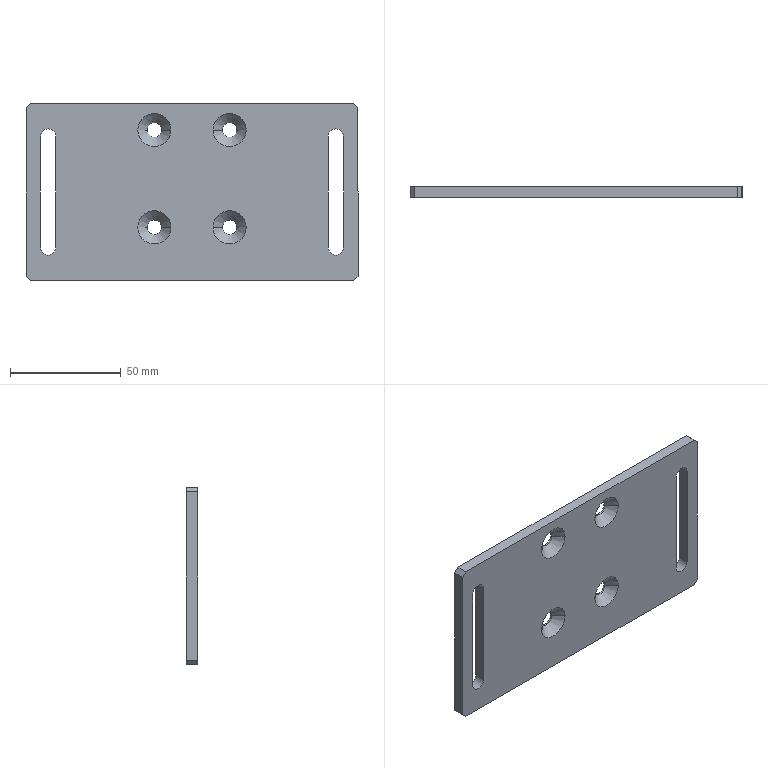Part | SolidWorks | features BaseBody 1 | 1 solid | 36 faces | box 150 x 5 x 80 mm | volume 54349 mm3 | cylinder 14 | plane 14 | cone 8 | commonest cylinder face diameters 6.6 x8 7 x6
STEP:
#1=CARTESIAN_POINT('',(10.,-5.,-11.5));
#2=VERTEX_POINT('',#1);
#3=CARTESIAN_POINT('',(13.5,-5.,-15.));
#4=VERTEX_POINT('',#3);
#5=CARTESIAN_POINT('',(10.,-5.,-15.));
#6=DIRECTION('',(0.,1.,0.));
#7=DIRECTION('',(0.,0.,1.));
#8=AXIS2_PLACEMENT_3D('',#5,#6,#7);
#9=CIRCLE('',#8,3.5);
#10=EDGE_CURVE('',#2,#4,#9,.T.);
#11=ORIENTED_EDGE('',*,*,#10,.F.);
#12=CARTESIAN_POINT('',(10.,0.,-11.5));
#13=VERTEX_POINT('',#12);
#14=CARTESIAN_POINT('',(10.,-10.,-11.5));
#15=DIRECTION('',(0.,1.,0.));
#16=VECTOR('',#15,1000.);
#17=LINE('',#14,#16);
#18=EDGE_CURVE('',#2,#13,#17,.T.);
#19=ORIENTED_EDGE('',*,*,#18,.T.);
#20=CARTESIAN_POINT('',(13.5,0.,-15.));
#21=VERTEX_POINT('',#20);
#22=CARTESIAN_POINT('',(10.,0.,-15.));
#23=DIRECTION('',(0.,1.,0.));
#24=DIRECTION('',(0.,0.,1.));
#25=AXIS2_PLACEMENT_3D('',#22,#23,#24);
#26=CIRCLE('',#25,3.5);
#27=EDGE_CURVE('',#13,#21,#26,.T.);
#28=ORIENTED_EDGE('',*,*,#27,.T.);
#29=CARTESIAN_POINT('',(13.5,-10.,-15.));
#30=DIRECTION('',(0.,-1.,0.));
#31=VECTOR('',#30,1000.);
#32=LINE('',#29,#31);
#33=EDGE_CURVE('',#21,#4,#32,.T.);
#34=ORIENTED_EDGE('',*,*,#33,.T.);
#35=EDGE_LOOP('',(#11,#19,#28,#34));
#36=FACE_OUTER_BOUND('',#35,.T.);
#37=CARTESIAN_POINT('',(10.,-10.,-15.));
#38=DIRECTION('',(0.,1.,0.));
#39=DIRECTION('',(0.,0.,1.));
#40=AXIS2_PLACEMENT_3D('',#37,#38,#39);
#41=CYLINDRICAL_SURFACE('',#40,3.5);
#42=ADVANCED_FACE('',(#36),#41,.F.);
#43=CARTESIAN_POINT('',(140.,-5.,-11.5));
#44=VERTEX_POINT('',#43);
#45=CARTESIAN_POINT('',(143.5,-5.,-15.));
#46=VERTEX_POINT('',#45);
#47=CARTESIAN_POINT('',(140.,-5.,-15.));
#48=DIRECTION('',(0.,1.,0.));
#49=DIRECTION('',(0.,0.,1.));
#50=AXIS2_PLACEMENT_3D('',#47,#48,#49);
#51=CIRCLE('',#50,3.5);
#52=EDGE_CURVE('',#44,#46,#51,.T.);
#53=ORIENTED_EDGE('',*,*,#52,.F.);
#54=CARTESIAN_POINT('',(140.,0.,-11.5));
#55=VERTEX_POINT('',#54);
#56=CARTESIAN_POINT('',(140.,-10.,-11.5));
#57=DIRECTION('',(0.,1.,0.));
#58=VECTOR('',#57,1000.);
#59=LINE('',#56,#58);
#60=EDGE_CURVE('',#44,#55,#59,.T.);
#61=ORIENTED_EDGE('',*,*,#60,.T.);
#62=CARTESIAN_POINT('',(143.5,0.,-15.));
#63=VERTEX_POINT('',#62);
#64=CARTESIAN_POINT('',(140.,0.,-15.));
#65=DIRECTION('',(0.,1.,0.));
#66=DIRECTION('',(0.,0.,1.));
#67=AXIS2_PLACEMENT_3D('',#64,#65,#66);
#68=CIRCLE('',#67,3.5);
#69=EDGE_CURVE('',#55,#63,#68,.T.);
#70=ORIENTED_EDGE('',*,*,#69,.T.);
#71=CARTESIAN_POINT('',(143.5,-10.,-15.));
#72=DIRECTION('',(0.,-1.,0.));
#73=VECTOR('',#72,1000.);
#74=LINE('',#71,#73);
#75=EDGE_CURVE('',#63,#46,#74,.T.);
#76=ORIENTED_EDGE('',*,*,#75,.T.);
#77=EDGE_LOOP('',(#53,#61,#70,#76));
#78=FACE_OUTER_BOUND('',#77,.T.);
#79=CARTESIAN_POINT('',(140.,-10.,-15.));
#80=DIRECTION('',(0.,1.,0.));
#81=DIRECTION('',(0.,0.,1.));
#82=AXIS2_PLACEMENT_3D('',#79,#80,#81);
#83=CYLINDRICAL_SURFACE('',#82,3.5);
#84=ADVANCED_FACE('',(#78),#83,.F.);
#85=CARTESIAN_POINT('',(92.,0.,-59.3));
#86=VERTEX_POINT('',#85);
#87=CARTESIAN_POINT('',(92.,0.,-52.7));
#88=VERTEX_POINT('',#87);
#89=CARTESIAN_POINT('',(92.,0.,-56.));
#90=DIRECTION('',(0.,1.,0.));
#91=DIRECTION('',(0.,0.,-1.));
#92=AXIS2_PLACEMENT_3D('',#89,#90,#91);
#93=CIRCLE('',#92,3.3);
#94=EDGE_CURVE('',#86,#88,#93,.T.);
#95=ORIENTED_EDGE('',*,*,#94,.T.);
#96=CARTESIAN_POINT('',(92.,-0.8,-52.7));
#97=VERTEX_POINT('',#96);
#98=CARTESIAN_POINT('',(92.,-5.,-52.7));
#99=DIRECTION('',(0.,-1.,0.));
#100=VECTOR('',#99,1000.);
#101=LINE('',#98,#100);
#102=EDGE_CURVE('',#88,#97,#101,.T.);
#103=ORIENTED_EDGE('',*,*,#102,.T.);
#104=CARTESIAN_POINT('',(88.7,-0.8,-56.));
#105=VERTEX_POINT('',#104);
#106=CARTESIAN_POINT('',(92.,-0.8,-56.));
#107=DIRECTION('',(0.,1.,0.));
#108=DIRECTION('',(0.,0.,-1.));
#109=AXIS2_PLACEMENT_3D('',#106,#107,#108);
#110=CIRCLE('',#109,3.3);
#111=EDGE_CURVE('',#105,#97,#110,.T.);
#112=ORIENTED_EDGE('',*,*,#111,.F.);
#113=CARTESIAN_POINT('',(92.,-0.8,-59.3));
#114=VERTEX_POINT('',#113);
#115=CARTESIAN_POINT('',(92.,-0.8,-56.));
#116=DIRECTION('',(0.,1.,0.));
#117=DIRECTION('',(0.,0.,-1.));
#118=AXIS2_PLACEMENT_3D('',#115,#116,#117);
#119=CIRCLE('',#118,3.3);
#120=EDGE_CURVE('',#114,#105,#119,.T.);
#121=ORIENTED_EDGE('',*,*,#120,.F.);
#122=CARTESIAN_POINT('',(92.,-5.,-59.3));
#123=DIRECTION('',(0.,-1.,0.));
#124=VECTOR('',#123,1000.);
#125=LINE('',#122,#124);
#126=EDGE_CURVE('',#86,#114,#125,.T.);
#127=ORIENTED_EDGE('',*,*,#126,.F.);
#128=EDGE_LOOP('',(#95,#103,#112,#121,#127));
#129=FACE_OUTER_BOUND('',#128,.T.);
#130=CARTESIAN_POINT('',(92.,-5.,-56.));
#131=DIRECTION('',(0.,-1.,0.));
#132=DIRECTION('',(0.,0.,-1.));
#133=AXIS2_PLACEMENT_3D('',#130,#131,#132);
#134=CYLINDRICAL_SURFACE('',#133,3.3);
#135=ADVANCED_FACE('',(#129),#134,.F.);
#136=CARTESIAN_POINT('',(92.,0.,-15.3));
#137=VERTEX_POINT('',#136);
#138=CARTESIAN_POINT('',(92.,0.,-8.7));
#139=VERTEX_POINT('',#138);
#140=CARTESIAN_POINT('',(92.,0.,-12.));
#141=DIRECTION('',(0.,1.,0.));
#142=DIRECTION('',(0.,0.,-1.));
#143=AXIS2_PLACEMENT_3D('',#140,#141,#142);
#144=CIRCLE('',#143,3.3);
#145=EDGE_CURVE('',#137,#139,#144,.T.);
#146=ORIENTED_EDGE('',*,*,#145,.T.);
#147=CARTESIAN_POINT('',(92.,-0.8,-8.7));
#148=VERTEX_POINT('',#147);
#149=CARTESIAN_POINT('',(92.,-5.,-8.7));
#150=DIRECTION('',(0.,-1.,0.));
#151=VECTOR('',#150,1000.);
#152=LINE('',#149,#151);
#153=EDGE_CURVE('',#139,#148,#152,.T.);
#154=ORIENTED_EDGE('',*,*,#153,.T.);
#155=CARTESIAN_POINT('',(88.7,-0.8,-12.));
#156=VERTEX_POINT('',#155);
#157=CARTESIAN_POINT('',(92.,-0.8,-12.));
#158=DIRECTION('',(0.,1.,0.));
#159=DIRECTION('',(0.,0.,-1.));
#160=AXIS2_PLACEMENT_3D('',#157,#158,#159);
#161=CIRCLE('',#160,3.3);
#162=EDGE_CURVE('',#156,#148,#161,.T.);
#163=ORIENTED_EDGE('',*,*,#162,.F.);
#164=CARTESIAN_POINT('',(92.,-0.8,-15.3));
#165=VERTEX_POINT('',#164);
#166=CARTESIAN_POINT('',(92.,-0.8,-12.));
#167=DIRECTION('',(0.,1.,0.));
#168=DIRECTION('',(0.,0.,-1.));
#169=AXIS2_PLACEMENT_3D('',#166,#167,#168);
#170=CIRCLE('',#169,3.3);
#171=EDGE_CURVE('',#165,#156,#170,.T.);
#172=ORIENTED_EDGE('',*,*,#171,.F.);
#173=CARTESIAN_POINT('',(92.,-5.,-15.3));
#174=DIRECTION('',(0.,-1.,0.));
#175=VECTOR('',#174,1000.);
#176=LINE('',#173,#175);
#177=EDGE_CURVE('',#137,#165,#176,.T.);
#178=ORIENTED_EDGE('',*,*,#177,.F.);
#179=EDGE_LOOP('',(#146,#154,#163,#172,#178));
#180=FACE_OUTER_BOUND('',#179,.T.);
#181=CARTESIAN_POINT('',(92.,-5.,-12.));
#182=DIRECTION('',(0.,-1.,0.));
#183=DIRECTION('',(0.,0.,-1.));
#184=AXIS2_PLACEMENT_3D('',#181,#182,#183);
#185=CYLINDRICAL_SURFACE('',#184,3.3);
#186=ADVANCED_FACE('',(#180),#185,.F.);
#187=CARTESIAN_POINT('',(58.,0.,-59.3));
#188=VERTEX_POINT('',#187);
#189=CARTESIAN_POINT('',(58.,0.,-52.7));
#190=VERTEX_POINT('',#189);
#191=CARTESIAN_POINT('',(58.,0.,-56.));
#192=DIRECTION('',(0.,1.,0.));
#193=DIRECTION('',(0.,0.,-1.));
#194=AXIS2_PLACEMENT_3D('',#191,#192,#193);
#195=CIRCLE('',#194,3.3);
#196=EDGE_CURVE('',#188,#190,#195,.T.);
#197=ORIENTED_EDGE('',*,*,#196,.T.);
#198=CARTESIAN_POINT('',(58.,-0.8,-52.7));
#199=VERTEX_POINT('',#198);
#200=CARTESIAN_POINT('',(58.,-5.,-52.7));
#201=DIRECTION('',(0.,-1.,0.));
#202=VECTOR('',#201,1000.);
#203=LINE('',#200,#202);
#204=EDGE_CURVE('',#190,#199,#203,.T.);
#205=ORIENTED_EDGE('',*,*,#204,.T.);
#206=CARTESIAN_POINT('',(54.7,-0.8,-56.));
#207=VERTEX_POINT('',#206);
#208=CARTESIAN_POINT('',(58.,-0.8,-56.));
#209=DIRECTION('',(0.,1.,0.));
#210=DIRECTION('',(0.,0.,-1.));
#211=AXIS2_PLACEMENT_3D('',#208,#209,#210);
#212=CIRCLE('',#211,3.3);
#213=EDGE_CURVE('',#207,#199,#212,.T.);
#214=ORIENTED_EDGE('',*,*,#213,.F.);
#215=CARTESIAN_POINT('',(58.,-0.8,-59.3));
#216=VERTEX_POINT('',#215);
#217=CARTESIAN_POINT('',(58.,-0.8,-56.));
#218=DIRECTION('',(0.,1.,0.));
#219=DIRECTION('',(0.,0.,-1.));
#220=AXIS2_PLACEMENT_3D('',#217,#218,#219);
#221=CIRCLE('',#220,3.3);
#222=EDGE_CURVE('',#216,#207,#221,.T.);
#223=ORIENTED_EDGE('',*,*,#222,.F.);
#224=CARTESIAN_POINT('',(58.,-5.,-59.3));
#225=DIRECTION('',(0.,-1.,0.));
#226=VECTOR('',#225,1000.);
#227=LINE('',#224,#226);
#228=EDGE_CURVE('',#188,#216,#227,.T.);
#229=ORIENTED_EDGE('',*,*,#228,.F.);
#230=EDGE_LOOP('',(#197,#205,#214,#223,#229));
#231=FACE_OUTER_BOUND('',#230,.T.);
#232=CARTESIAN_POINT('',(58.,-5.,-56.));
#233=DIRECTION('',(0.,-1.,0.));
#234=DIRECTION('',(0.,0.,-1.));
#235=AXIS2_PLACEMENT_3D('',#232,#233,#234);
#236=CYLINDRICAL_SURFACE('',#235,3.3);
#237=ADVANCED_FACE('',(#231),#236,.F.);
#238=CARTESIAN_POINT('',(58.,0.,-15.3));
#239=VERTEX_POINT('',#238);
#240=CARTESIAN_POINT('',(58.,0.,-8.7));
#241=VERTEX_POINT('',#240);
#242=CARTESIAN_POINT('',(58.,0.,-12.));
#243=DIRECTION('',(0.,1.,0.));
#244=DIRECTION('',(0.,0.,-1.));
#245=AXIS2_PLACEMENT_3D('',#242,#243,#244);
#246=CIRCLE('',#245,3.3);
#247=EDGE_CURVE('',#239,#241,#246,.T.);
#248=ORIENTED_EDGE('',*,*,#247,.T.);
#249=CARTESIAN_POINT('',(58.,-0.8,-8.7));
#250=VERTEX_POINT('',#249);
#251=CARTESIAN_POINT('',(58.,-5.,-8.7));
#252=DIRECTION('',(0.,-1.,0.));
#253=VECTOR('',#252,1000.);
#254=LINE('',#251,#253);
#255=EDGE_CURVE('',#241,#250,#254,.T.);
#256=ORIENTED_EDGE('',*,*,#255,.T.);
#257=CARTESIAN_POINT('',(54.7,-0.8,-12.));
#258=VERTEX_POINT('',#257);
#259=CARTESIAN_POINT('',(58.,-0.8,-12.));
#260=DIRECTION('',(0.,1.,0.));
#261=DIRECTION('',(0.,0.,-1.));
#262=AXIS2_PLACEMENT_3D('',#259,#260,#261);
#263=CIRCLE('',#262,3.3);
#264=EDGE_CURVE('',#258,#250,#263,.T.);
#265=ORIENTED_EDGE('',*,*,#264,.F.);
#266=CARTESIAN_POINT('',(58.,-0.8,-15.3));
#267=VERTEX_POINT('',#266);
#268=CARTESIAN_POINT('',(58.,-0.8,-12.));
#269=DIRECTION('',(0.,1.,0.));
#270=DIRECTION('',(0.,0.,-1.));
#271=AXIS2_PLACEMENT_3D('',#268,#269,#270);
#272=CIRCLE('',#271,3.3);
#273=EDGE_CURVE('',#267,#258,#272,.T.);
#274=ORIENTED_EDGE('',*,*,#273,.F.);
#275=CARTESIAN_POINT('',(58.,-5.,-15.3));
#276=DIRECTION('',(0.,-1.,0.));
#277=VECTOR('',#276,1000.);
#278=LINE('',#275,#277);
#279=EDGE_CURVE('',#239,#267,#278,.T.);
#280=ORIENTED_EDGE('',*,*,#279,.F.);
#281=EDGE_LOOP('',(#248,#256,#265,#274,#280));
#282=FACE_OUTER_BOUND('',#281,.T.);
#283=CARTESIAN_POINT('',(58.,-5.,-12.));
#284=DIRECTION('',(0.,-1.,0.));
#285=DIRECTION('',(0.,0.,-1.));
#286=AXIS2_PLACEMENT_3D('',#283,#284,#285);
#287=CYLINDRICAL_SURFACE('',#286,3.3);
#288=ADVANCED_FACE('',(#282),#287,.F.);
#289=CARTESIAN_POINT('',(95.3,-0.8,-56.));
#290=VERTEX_POINT('',#289);
#291=CARTESIAN_POINT('',(92.,-0.8,-56.));
#292=DIRECTION('',(0.,1.,0.));
#293=DIRECTION('',(0.,0.,-1.));
#294=AXIS2_PLACEMENT_3D('',#291,#292,#293);
#295=CIRCLE('',#294,3.3);
#296=EDGE_CURVE('',#290,#114,#295,.T.);
#297=ORIENTED_EDGE('',*,*,#296,.T.);
#298=ORIENTED_EDGE('',*,*,#120,.T.);
#299=CARTESIAN_POINT('',(84.5,-5.,-56.));
#300=VERTEX_POINT('',#299);
#301=CARTESIAN_POINT('',(84.5,-5.,-56.));
#302=DIRECTION('',(-0.7071,-0.7071,0.));
#303=VECTOR('',#302,1000.);
#304=LINE('',#301,#303);
#305=EDGE_CURVE('',#105,#300,#304,.T.);
#306=ORIENTED_EDGE('',*,*,#305,.T.);
#307=CARTESIAN_POINT('',(99.5,-5.,-56.));
#308=VERTEX_POINT('',#307);
#309=CARTESIAN_POINT('',(92.,-5.,-56.));
#310=DIRECTION('',(0.,1.,0.));
#311=DIRECTION('',(1.,0.,0.));
#312=AXIS2_PLACEMENT_3D('',#309,#310,#311);
#313=CIRCLE('',#312,7.5);
#314=EDGE_CURVE('',#308,#300,#313,.T.);
#315=ORIENTED_EDGE('',*,*,#314,.F.);
#316=CARTESIAN_POINT('',(99.5,-5.,-56.));
#317=DIRECTION('',(0.7071,-0.7071,0.));
#318=VECTOR('',#317,1000.);
#319=LINE('',#316,#318);
#320=EDGE_CURVE('',#290,#308,#319,.T.);
#321=ORIENTED_EDGE('',*,*,#320,.F.);
#322=EDGE_LOOP('',(#297,#298,#306,#315,#321));
#323=FACE_OUTER_BOUND('',#322,.T.);
#324=CARTESIAN_POINT('',(92.,-5.,-56.));
#325=DIRECTION('',(0.,-1.,0.));
#326=DIRECTION('',(1.,0.,0.));
#327=AXIS2_PLACEMENT_3D('',#324,#325,#326);
#328=CONICAL_SURFACE('',#327,7.5,0.7854);
#329=ADVANCED_FACE('',(#323),#328,.F.);
#330=CARTESIAN_POINT('',(95.3,-0.8,-12.));
#331=VERTEX_POINT('',#330);
#332=CARTESIAN_POINT('',(92.,-0.8,-12.));
#333=DIRECTION('',(0.,1.,0.));
#334=DIRECTION('',(0.,0.,-1.));
#335=AXIS2_PLACEMENT_3D('',#332,#333,#334);
#336=CIRCLE('',#335,3.3);
#337=EDGE_CURVE('',#331,#165,#336,.T.);
#338=ORIENTED_EDGE('',*,*,#337,.T.);
#339=ORIENTED_EDGE('',*,*,#171,.T.);
#340=CARTESIAN_POINT('',(84.5,-5.,-12.));
#341=VERTEX_POINT('',#340);
#342=CARTESIAN_POINT('',(84.5,-5.,-12.));
#343=DIRECTION('',(-0.7071,-0.7071,0.));
#344=VECTOR('',#343,1000.);
#345=LINE('',#342,#344);
#346=EDGE_CURVE('',#156,#341,#345,.T.);
#347=ORIENTED_EDGE('',*,*,#346,.T.);
#348=CARTESIAN_POINT('',(99.5,-5.,-12.));
#349=VERTEX_POINT('',#348);
#350=CARTESIAN_POINT('',(92.,-5.,-12.));
#351=DIRECTION('',(0.,1.,0.));
#352=DIRECTION('',(1.,0.,0.));
#353=AXIS2_PLACEMENT_3D('',#350,#351,#352);
#354=CIRCLE('',#353,7.5);
#355=EDGE_CURVE('',#349,#341,#354,.T.);
#356=ORIENTED_EDGE('',*,*,#355,.F.);
#357=CARTESIAN_POINT('',(99.5,-5.,-12.));
#358=DIRECTION('',(0.7071,-0.7071,0.));
#359=VECTOR('',#358,1000.);
#360=LINE('',#357,#359);
#361=EDGE_CURVE('',#331,#349,#360,.T.);
#362=ORIENTED_EDGE('',*,*,#361,.F.);
#363=EDGE_LOOP('',(#338,#339,#347,#356,#362));
#364=FACE_OUTER_BOUND('',#363,.T.);
#365=CARTESIAN_POINT('',(92.,-5.,-12.));
#366=DIRECTION('',(0.,-1.,0.));
#367=DIRECTION('',(1.,0.,0.));
#368=AXIS2_PLACEMENT_3D('',#365,#366,#367);
#369=CONICAL_SURFACE('',#368,7.5,0.7854);
#370=ADVANCED_FACE('',(#364),#369,.F.);
#371=CARTESIAN_POINT('',(61.3,-0.8,-56.));
#372=VERTEX_POINT('',#371);
#373=CARTESIAN_POINT('',(58.,-0.8,-56.));
#374=DIRECTION('',(0.,1.,0.));
#375=DIRECTION('',(0.,0.,-1.));
#376=AXIS2_PLACEMENT_3D('',#373,#374,#375);
#377=CIRCLE('',#376,3.3);
#378=EDGE_CURVE('',#372,#216,#377,.T.);
#379=ORIENTED_EDGE('',*,*,#378,.T.);
#380=ORIENTED_EDGE('',*,*,#222,.T.);
#381=CARTESIAN_POINT('',(50.5,-5.,-56.));
#382=VERTEX_POINT('',#381);
#383=CARTESIAN_POINT('',(50.5,-5.,-56.));
#384=DIRECTION('',(-0.7071,-0.7071,0.));
#385=VECTOR('',#384,1000.);
#386=LINE('',#383,#385);
#387=EDGE_CURVE('',#207,#382,#386,.T.);
#388=ORIENTED_EDGE('',*,*,#387,.T.);
#389=CARTESIAN_POINT('',(65.5,-5.,-56.));
#390=VERTEX_POINT('',#389);
#391=CARTESIAN_POINT('',(58.,-5.,-56.));
#392=DIRECTION('',(0.,1.,0.));
#393=DIRECTION('',(1.,0.,0.));
#394=AXIS2_PLACEMENT_3D('',#391,#392,#393);
#395=CIRCLE('',#394,7.5);
#396=EDGE_CURVE('',#390,#382,#395,.T.);
#397=ORIENTED_EDGE('',*,*,#396,.F.);
#398=CARTESIAN_POINT('',(65.5,-5.,-56.));
#399=DIRECTION('',(0.7071,-0.7071,0.));
#400=VECTOR('',#399,1000.);
#401=LINE('',#398,#400);
#402=EDGE_CURVE('',#372,#390,#401,.T.);
#403=ORIENTED_EDGE('',*,*,#402,.F.);
#404=EDGE_LOOP('',(#379,#380,#388,#397,#403));
#405=FACE_OUTER_BOUND('',#404,.T.);
#406=CARTESIAN_POINT('',(58.,-5.,-56.));
#407=DIRECTION('',(0.,-1.,0.));
#408=DIRECTION('',(1.,0.,0.));
#409=AXIS2_PLACEMENT_3D('',#406,#407,#408);
#410=CONICAL_SURFACE('',#409,7.5,0.7854);
#411=ADVANCED_FACE('',(#405),#410,.F.);
#412=CARTESIAN_POINT('',(61.3,-0.8,-12.));
#413=VERTEX_POINT('',#412);
#414=CARTESIAN_POINT('',(58.,-0.8,-12.));
#415=DIRECTION('',(0.,1.,0.));
#416=DIRECTION('',(0.,0.,-1.));
#417=AXIS2_PLACEMENT_3D('',#414,#415,#416);
#418=CIRCLE('',#417,3.3);
#419=EDGE_CURVE('',#413,#267,#418,.T.);
#420=ORIENTED_EDGE('',*,*,#419,.T.);
#421=ORIENTED_EDGE('',*,*,#273,.T.);
#422=CARTESIAN_POINT('',(50.5,-5.,-12.));
#423=VERTEX_POINT('',#422);
#424=CARTESIAN_POINT('',(50.5,-5.,-12.));
#425=DIRECTION('',(-0.7071,-0.7071,0.));
#426=VECTOR('',#425,1000.);
#427=LINE('',#424,#426);
#428=EDGE_CURVE('',#258,#423,#427,.T.);
#429=ORIENTED_EDGE('',*,*,#428,.T.);
#430=CARTESIAN_POINT('',(65.5,-5.,-12.));
#431=VERTEX_POINT('',#430);
#432=CARTESIAN_POINT('',(58.,-5.,-12.));
#433=DIRECTION('',(0.,1.,0.));
#434=DIRECTION('',(1.,0.,0.));
#435=AXIS2_PLACEMENT_3D('',#432,#433,#434);
#436=CIRCLE('',#435,7.5);
#437=EDGE_CURVE('',#431,#423,#436,.T.);
#438=ORIENTED_EDGE('',*,*,#437,.F.);
#439=CARTESIAN_POINT('',(65.5,-5.,-12.));
#440=DIRECTION('',(0.7071,-0.7071,0.));
#441=VECTOR('',#440,1000.);
#442=LINE('',#439,#441);
#443=EDGE_CURVE('',#413,#431,#442,.T.);
#444=ORIENTED_EDGE('',*,*,#443,.F.);
#445=EDGE_LOOP('',(#420,#421,#429,#438,#444));
#446=FACE_OUTER_BOUND('',#445,.T.);
#447=CARTESIAN_POINT('',(58.,-5.,-12.));
#448=DIRECTION('',(0.,-1.,0.));
#449=DIRECTION('',(1.,0.,0.));
#450=AXIS2_PLACEMENT_3D('',#447,#448,#449);
#451=CONICAL_SURFACE('',#450,7.5,0.7854);
#452=ADVANCED_FACE('',(#446),#451,.F.);
#453=CARTESIAN_POINT('',(0.,0.,-78.));
#454=VERTEX_POINT('',#453);
#455=CARTESIAN_POINT('',(2.,0.,-80.));
#456=VERTEX_POINT('',#455);
#457=CARTESIAN_POINT('',(0.,0.,-78.));
#458=DIRECTION('',(0.7071,0.,-0.7071));
#459=VECTOR('',#458,1000.);
#460=LINE('',#457,#459);
#461=EDGE_CURVE('',#454,#456,#460,.T.);
#462=ORIENTED_EDGE('',*,*,#461,.F.);
#463=CARTESIAN_POINT('',(0.,0.,-2.));
#464=VERTEX_POINT('',#463);
#465=CARTESIAN_POINT('',(0.,0.,0.));
#466=DIRECTION('',(0.,0.,-1.));
#467=VECTOR('',#466,1000.);
#468=LINE('',#465,#467);
#469=EDGE_CURVE('',#464,#454,#468,.T.);
#470=ORIENTED_EDGE('',*,*,#469,.F.);
#471=CARTESIAN_POINT('',(2.,0.,0.));
#472=VERTEX_POINT('',#471);
#473=CARTESIAN_POINT('',(2.,0.,0.));
#474=DIRECTION('',(-0.7071,0.,-0.7071));
#475=VECTOR('',#474,1000.);
#476=LINE('',#473,#475);
#477=EDGE_CURVE('',#472,#464,#476,.T.);
#478=ORIENTED_EDGE('',*,*,#477,.F.);
#479=CARTESIAN_POINT('',(148.,0.,0.));
#480=VERTEX_POINT('',#479);
#481=CARTESIAN_POINT('',(0.,0.,0.));
#482=DIRECTION('',(-1.,0.,0.));
#483=VECTOR('',#482,1000.);
#484=LINE('',#481,#483);
#485=EDGE_CURVE('',#480,#472,#484,.T.);
#486=ORIENTED_EDGE('',*,*,#485,.F.);
#487=CARTESIAN_POINT('',(150.,0.,-2.));
#488=VERTEX_POINT('',#487);
#489=CARTESIAN_POINT('',(150.,0.,-2.));
#490=DIRECTION('',(-0.7071,0.,0.7071));
#491=VECTOR('',#490,1000.);
#492=LINE('',#489,#491);
#493=EDGE_CURVE('',#488,#480,#492,.T.);
#494=ORIENTED_EDGE('',*,*,#493,.F.);
#495=CARTESIAN_POINT('',(150.,0.,-78.));
#496=VERTEX_POINT('',#495);
#497=CARTESIAN_POINT('',(150.,0.,0.));
#498=DIRECTION('',(0.,0.,1.));
#499=VECTOR('',#498,1000.);
#500=LINE('',#497,#499);
#501=EDGE_CURVE('',#496,#488,#500,.T.);
#502=ORIENTED_EDGE('',*,*,#501,.F.);
#503=CARTESIAN_POINT('',(148.,0.,-80.));
#504=VERTEX_POINT('',#503);
#505=CARTESIAN_POINT('',(148.,0.,-80.));
#506=DIRECTION('',(0.7071,0.,0.7071));
#507=VECTOR('',#506,1000.);
#508=LINE('',#505,#507);
#509=EDGE_CURVE('',#504,#496,#508,.T.);
#510=ORIENTED_EDGE('',*,*,#509,.F.);
#511=CARTESIAN_POINT('',(0.,0.,-80.));
#512=DIRECTION('',(1.,0.,0.));
#513=VECTOR('',#512,1000.);
#514=LINE('',#511,#513);
#515=EDGE_CURVE('',#456,#504,#514,.T.);
#516=ORIENTED_EDGE('',*,*,#515,.F.);
#517=EDGE_LOOP('',(#462,#470,#478,#486,#494,#502,#510,#516));
#518=FACE_OUTER_BOUND('',#517,.T.);
#519=CARTESIAN_POINT('',(13.5,0.,-65.));
#520=VERTEX_POINT('',#519);
#521=CARTESIAN_POINT('',(6.5,0.,-65.));
#522=VERTEX_POINT('',#521);
#523=CARTESIAN_POINT('',(10.,0.,-65.));
#524=DIRECTION('',(0.,1.,0.));
#525=DIRECTION('',(0.,0.,1.));
#526=AXIS2_PLACEMENT_3D('',#523,#524,#525);
#527=CIRCLE('',#526,3.5);
#528=EDGE_CURVE('',#520,#522,#527,.T.);
#529=ORIENTED_EDGE('',*,*,#528,.F.);
#530=CARTESIAN_POINT('',(13.5,0.,0.));
#531=DIRECTION('',(0.,0.,-1.));
#532=VECTOR('',#531,1000.);
#533=LINE('',#530,#532);
#534=EDGE_CURVE('',#21,#520,#533,.T.);
#535=ORIENTED_EDGE('',*,*,#534,.F.);
#536=ORIENTED_EDGE('',*,*,#27,.F.);
#537=CARTESIAN_POINT('',(6.5,0.,-15.));
#538=VERTEX_POINT('',#537);
#539=CARTESIAN_POINT('',(10.,0.,-15.));
#540=DIRECTION('',(0.,1.,0.));
#541=DIRECTION('',(0.,0.,1.));
#542=AXIS2_PLACEMENT_3D('',#539,#540,#541);
#543=CIRCLE('',#542,3.5);
#544=EDGE_CURVE('',#538,#13,#543,.T.);
#545=ORIENTED_EDGE('',*,*,#544,.F.);
#546=CARTESIAN_POINT('',(6.5,0.,0.));
#547=DIRECTION('',(0.,0.,1.));
#548=VECTOR('',#547,1000.);
#549=LINE('',#546,#548);
#550=EDGE_CURVE('',#522,#538,#549,.T.);
#551=ORIENTED_EDGE('',*,*,#550,.F.);
#552=EDGE_LOOP('',(#529,#535,#536,#545,#551));
#553=FACE_BOUND('',#552,.T.);
#554=CARTESIAN_POINT('',(143.5,0.,-65.));
#555=VERTEX_POINT('',#554);
#556=CARTESIAN_POINT('',(136.5,0.,-65.));
#557=VERTEX_POINT('',#556);
#558=CARTESIAN_POINT('',(140.,0.,-65.));
#559=DIRECTION('',(0.,1.,0.));
#560=DIRECTION('',(0.,0.,1.));
#561=AXIS2_PLACEMENT_3D('',#558,#559,#560);
#562=CIRCLE('',#561,3.5);
#563=EDGE_CURVE('',#555,#557,#562,.T.);
#564=ORIENTED_EDGE('',*,*,#563,.F.);
#565=CARTESIAN_POINT('',(143.5,0.,0.));
#566=DIRECTION('',(0.,0.,-1.));
#567=VECTOR('',#566,1000.);
#568=LINE('',#565,#567);
#569=EDGE_CURVE('',#63,#555,#568,.T.);
#570=ORIENTED_EDGE('',*,*,#569,.F.);
#571=ORIENTED_EDGE('',*,*,#69,.F.);
#572=CARTESIAN_POINT('',(136.5,0.,-15.));
#573=VERTEX_POINT('',#572);
#574=CARTESIAN_POINT('',(140.,0.,-15.));
#575=DIRECTION('',(0.,1.,0.));
#576=DIRECTION('',(0.,0.,1.));
#577=AXIS2_PLACEMENT_3D('',#574,#575,#576);
#578=CIRCLE('',#577,3.5);
#579=EDGE_CURVE('',#573,#55,#578,.T.);
#580=ORIENTED_EDGE('',*,*,#579,.F.);
#581=CARTESIAN_POINT('',(136.5,0.,0.));
#582=DIRECTION('',(0.,0.,1.));
#583=VECTOR('',#582,1000.);
#584=LINE('',#581,#583);
#585=EDGE_CURVE('',#557,#573,#584,.T.);
#586=ORIENTED_EDGE('',*,*,#585,.F.);
#587=EDGE_LOOP('',(#564,#570,#571,#580,#586));
#588=FACE_BOUND('',#587,.T.);
#589=ORIENTED_EDGE('',*,*,#94,.F.);
#590=CARTESIAN_POINT('',(92.,0.,-56.));
#591=DIRECTION('',(0.,1.,0.));
#592=DIRECTION('',(0.,0.,-1.));
#593=AXIS2_PLACEMENT_3D('',#590,#591,#592);
#594=CIRCLE('',#593,3.3);
#595=EDGE_CURVE('',#88,#86,#594,.T.);
#596=ORIENTED_EDGE('',*,*,#595,.F.);
#597=EDGE_LOOP('',(#589,#596));
#598=FACE_BOUND('',#597,.T.);
#599=ORIENTED_EDGE('',*,*,#145,.F.);
#600=CARTESIAN_POINT('',(92.,0.,-12.));
#601=DIRECTION('',(0.,1.,0.));
#602=DIRECTION('',(0.,0.,-1.));
#603=AXIS2_PLACEMENT_3D('',#600,#601,#602);
#604=CIRCLE('',#603,3.3);
#605=EDGE_CURVE('',#139,#137,#604,.T.);
#606=ORIENTED_EDGE('',*,*,#605,.F.);
#607=EDGE_LOOP('',(#599,#606));
#608=FACE_BOUND('',#607,.T.);
#609=ORIENTED_EDGE('',*,*,#196,.F.);
#610=CARTESIAN_POINT('',(58.,0.,-56.));
#611=DIRECTION('',(0.,1.,0.));
#612=DIRECTION('',(0.,0.,-1.));
#613=AXIS2_PLACEMENT_3D('',#610,#611,#612);
#614=CIRCLE('',#613,3.3);
#615=EDGE_CURVE('',#190,#188,#614,.T.);
#616=ORIENTED_EDGE('',*,*,#615,.F.);
#617=EDGE_LOOP('',(#609,#616));
#618=FACE_BOUND('',#617,.T.);
#619=ORIENTED_EDGE('',*,*,#247,.F.);
#620=CARTESIAN_POINT('',(58.,0.,-12.));
#621=DIRECTION('',(0.,1.,0.));
#622=DIRECTION('',(0.,0.,-1.));
#623=AXIS2_PLACEMENT_3D('',#620,#621,#622);
#624=CIRCLE('',#623,3.3);
#625=EDGE_CURVE('',#241,#239,#624,.T.);
#626=ORIENTED_EDGE('',*,*,#625,.F.);
#627=EDGE_LOOP('',(#619,#626));
#628=FACE_BOUND('',#627,.T.);
#629=CARTESIAN_POINT('',(0.,0.,0.));
#630=DIRECTION('',(0.,-1.,0.));
#631=DIRECTION('',(0.,0.,-1.));
#632=AXIS2_PLACEMENT_3D('',#629,#630,#631);
#633=PLANE('',#632);
#634=ADVANCED_FACE('',(#518,#553,#588,#598,#608,#618,#628),#633,.F.);
#635=ORIENTED_EDGE('',*,*,#515,.T.);
#636=CARTESIAN_POINT('',(148.,-5.,-80.));
#637=VERTEX_POINT('',#636);
#638=CARTESIAN_POINT('',(148.,-5.,-80.));
#639=DIRECTION('',(0.,-1.,0.));
#640=VECTOR('',#639,1000.);
#641=LINE('',#638,#640);
#642=EDGE_CURVE('',#504,#637,#641,.T.);
#643=ORIENTED_EDGE('',*,*,#642,.T.);
#644=CARTESIAN_POINT('',(2.,-5.,-80.));
#645=VERTEX_POINT('',#644);
#646=CARTESIAN_POINT('',(0.,-5.,-80.));
#647=DIRECTION('',(-1.,0.,0.));
#648=VECTOR('',#647,1000.);
#649=LINE('',#646,#648);
#650=EDGE_CURVE('',#637,#645,#649,.T.);
#651=ORIENTED_EDGE('',*,*,#650,.T.);
#652=CARTESIAN_POINT('',(2.,-5.,-80.));
#653=DIRECTION('',(0.,1.,0.));
#654=VECTOR('',#653,1000.);
#655=LINE('',#652,#654);
#656=EDGE_CURVE('',#645,#456,#655,.T.);
#657=ORIENTED_EDGE('',*,*,#656,.T.);
#658=EDGE_LOOP('',(#635,#643,#651,#657));
#659=FACE_OUTER_BOUND('',#658,.T.);
#660=CARTESIAN_POINT('',(0.,-5.,-80.));
#661=DIRECTION('',(0.,0.,-1.));
#662=DIRECTION('',(-1.,0.,0.));
#663=AXIS2_PLACEMENT_3D('',#660,#661,#662);
#664=PLANE('',#663);
#665=ADVANCED_FACE('',(#659),#664,.T.);
#666=CARTESIAN_POINT('',(0.,-5.,-78.));
#667=VERTEX_POINT('',#666);
#668=CARTESIAN_POINT('',(0.,-5.,-78.));
#669=DIRECTION('',(0.,-1.,0.));
#670=VECTOR('',#669,1000.);
#671=LINE('',#668,#670);
#672=EDGE_CURVE('',#454,#667,#671,.T.);
#673=ORIENTED_EDGE('',*,*,#672,.F.);
#674=ORIENTED_EDGE('',*,*,#461,.T.);
#675=ORIENTED_EDGE('',*,*,#656,.F.);
#676=CARTESIAN_POINT('',(2.,-5.,-80.));
#677=DIRECTION('',(0.7071,0.,-0.7071));
#678=VECTOR('',#677,1000.);
#679=LINE('',#676,#678);
#680=EDGE_CURVE('',#667,#645,#679,.T.);
#681=ORIENTED_EDGE('',*,*,#680,.F.);
#682=EDGE_LOOP('',(#673,#674,#675,#681));
#683=FACE_OUTER_BOUND('',#682,.T.);
#684=CARTESIAN_POINT('',(2.,-5.,-80.));
#685=DIRECTION('',(0.7071,0.,0.7071));
#686=DIRECTION('',(0.7071,0.,-0.7071));
#687=AXIS2_PLACEMENT_3D('',#684,#685,#686);
#688=PLANE('',#687);
#689=ADVANCED_FACE('',(#683),#688,.F.);
#690=CARTESIAN_POINT('',(0.,-5.,-2.));
#691=VERTEX_POINT('',#690);
#692=CARTESIAN_POINT('',(0.,-5.,0.));
#693=DIRECTION('',(0.,0.,1.));
#694=VECTOR('',#693,1000.);
#695=LINE('',#692,#694);
#696=EDGE_CURVE('',#667,#691,#695,.T.);
#697=ORIENTED_EDGE('',*,*,#696,.T.);
#698=CARTESIAN_POINT('',(0.,-5.,-2.));
#699=DIRECTION('',(0.,1.,0.));
#700=VECTOR('',#699,1000.);
#701=LINE('',#698,#700);
#702=EDGE_CURVE('',#691,#464,#701,.T.);
#703=ORIENTED_EDGE('',*,*,#702,.T.);
#704=ORIENTED_EDGE('',*,*,#469,.T.);
#705=ORIENTED_EDGE('',*,*,#672,.T.);
#706=EDGE_LOOP('',(#697,#703,#704,#705));
#707=FACE_OUTER_BOUND('',#706,.T.);
#708=CARTESIAN_POINT('',(0.,-5.,0.));
#709=DIRECTION('',(-1.,0.,0.));
#710=DIRECTION('',(0.,0.,1.));
#711=AXIS2_PLACEMENT_3D('',#708,#709,#710);
#712=PLANE('',#711);
#713=ADVANCED_FACE('',(#707),#712,.T.);
#714=CARTESIAN_POINT('',(2.,-5.,0.));
#715=VERTEX_POINT('',#714);
#716=CARTESIAN_POINT('',(2.,-5.,0.));
#717=DIRECTION('',(0.,-1.,0.));
#718=VECTOR('',#717,1000.);
#719=LINE('',#716,#718);
#720=EDGE_CURVE('',#472,#715,#719,.T.);
#721=ORIENTED_EDGE('',*,*,#720,.F.);
#722=ORIENTED_EDGE('',*,*,#477,.T.);
#723=ORIENTED_EDGE('',*,*,#702,.F.);
#724=CARTESIAN_POINT('',(0.,-5.,-2.));
#725=DIRECTION('',(-0.7071,0.,-0.7071));
#726=VECTOR('',#725,1000.);
#727=LINE('',#724,#726);
#728=EDGE_CURVE('',#715,#691,#727,.T.);
#729=ORIENTED_EDGE('',*,*,#728,.F.);
#730=EDGE_LOOP('',(#721,#722,#723,#729));
#731=FACE_OUTER_BOUND('',#730,.T.);
#732=CARTESIAN_POINT('',(0.,-5.,-2.));
#733=DIRECTION('',(0.7071,0.,-0.7071));
#734=DIRECTION('',(-0.7071,0.,-0.7071));
#735=AXIS2_PLACEMENT_3D('',#732,#733,#734);
#736=PLANE('',#735);
#737=ADVANCED_FACE('',(#731),#736,.F.);
#738=CARTESIAN_POINT('',(148.,-5.,0.));
#739=VERTEX_POINT('',#738);
#740=CARTESIAN_POINT('',(0.,-5.,0.));
#741=DIRECTION('',(1.,0.,0.));
#742=VECTOR('',#741,1000.);
#743=LINE('',#740,#742);
#744=EDGE_CURVE('',#715,#739,#743,.T.);
#745=ORIENTED_EDGE('',*,*,#744,.T.);
#746=CARTESIAN_POINT('',(148.,-5.,0.));
#747=DIRECTION('',(0.,1.,0.));
#748=VECTOR('',#747,1000.);
#749=LINE('',#746,#748);
#750=EDGE_CURVE('',#739,#480,#749,.T.);
#751=ORIENTED_EDGE('',*,*,#750,.T.);
#752=ORIENTED_EDGE('',*,*,#485,.T.);
#753=ORIENTED_EDGE('',*,*,#720,.T.);
#754=EDGE_LOOP('',(#745,#751,#752,#753));
#755=FACE_OUTER_BOUND('',#754,.T.);
#756=CARTESIAN_POINT('',(0.,-5.,0.));
#757=DIRECTION('',(0.,0.,1.));
#758=DIRECTION('',(1.,0.,0.));
#759=AXIS2_PLACEMENT_3D('',#756,#757,#758);
#760=PLANE('',#759);
#761=ADVANCED_FACE('',(#755),#760,.T.);
#762=CARTESIAN_POINT('',(150.,-5.,-2.));
#763=VERTEX_POINT('',#762);
#764=CARTESIAN_POINT('',(150.,-5.,-2.));
#765=DIRECTION('',(0.,-1.,0.));
#766=VECTOR('',#765,1000.);
#767=LINE('',#764,#766);
#768=EDGE_CURVE('',#488,#763,#767,.T.);
#769=ORIENTED_EDGE('',*,*,#768,.F.);
#770=ORIENTED_EDGE('',*,*,#493,.T.);
#771=ORIENTED_EDGE('',*,*,#750,.F.);
#772=CARTESIAN_POINT('',(148.,-5.,0.));
#773=DIRECTION('',(-0.7071,0.,0.7071));
#774=VECTOR('',#773,1000.);
#775=LINE('',#772,#774);
#776=EDGE_CURVE('',#763,#739,#775,.T.);
#777=ORIENTED_EDGE('',*,*,#776,.F.);
#778=EDGE_LOOP('',(#769,#770,#771,#777));
#779=FACE_OUTER_BOUND('',#778,.T.);
#780=CARTESIAN_POINT('',(148.,-5.,0.));
#781=DIRECTION('',(-0.7071,0.,-0.7071));
#782=DIRECTION('',(-0.7071,0.,0.7071));
#783=AXIS2_PLACEMENT_3D('',#780,#781,#782);
#784=PLANE('',#783);
#785=ADVANCED_FACE('',(#779),#784,.F.);
#786=ORIENTED_EDGE('',*,*,#501,.T.);
#787=ORIENTED_EDGE('',*,*,#768,.T.);
#788=CARTESIAN_POINT('',(150.,-5.,-78.));
#789=VERTEX_POINT('',#788);
#790=CARTESIAN_POINT('',(150.,-5.,0.));
#791=DIRECTION('',(0.,0.,-1.));
#792=VECTOR('',#791,1000.);
#793=LINE('',#790,#792);
#794=EDGE_CURVE('',#763,#789,#793,.T.);
#795=ORIENTED_EDGE('',*,*,#794,.T.);
#796=CARTESIAN_POINT('',(150.,-5.,-78.));
#797=DIRECTION('',(0.,1.,0.));
#798=VECTOR('',#797,1000.);
#799=LINE('',#796,#798);
#800=EDGE_CURVE('',#789,#496,#799,.T.);
#801=ORIENTED_EDGE('',*,*,#800,.T.);
#802=EDGE_LOOP('',(#786,#787,#795,#801));
#803=FACE_OUTER_BOUND('',#802,.T.);
#804=CARTESIAN_POINT('',(150.,-5.,0.));
#805=DIRECTION('',(1.,0.,0.));
#806=DIRECTION('',(0.,0.,-1.));
#807=AXIS2_PLACEMENT_3D('',#804,#805,#806);
#808=PLANE('',#807);
#809=ADVANCED_FACE('',(#803),#808,.T.);
#810=ORIENTED_EDGE('',*,*,#642,.F.);
#811=ORIENTED_EDGE('',*,*,#509,.T.);
#812=ORIENTED_EDGE('',*,*,#800,.F.);
#813=CARTESIAN_POINT('',(150.,-5.,-78.));
#814=DIRECTION('',(0.7071,0.,0.7071));
#815=VECTOR('',#814,1000.);
#816=LINE('',#813,#815);
#817=EDGE_CURVE('',#637,#789,#816,.T.);
#818=ORIENTED_EDGE('',*,*,#817,.F.);
#819=EDGE_LOOP('',(#810,#811,#812,#818));
#820=FACE_OUTER_BOUND('',#819,.T.);
#821=CARTESIAN_POINT('',(150.,-5.,-78.));
#822=DIRECTION('',(-0.7071,0.,0.7071));
#823=DIRECTION('',(0.7071,0.,0.7071));
#824=AXIS2_PLACEMENT_3D('',#821,#822,#823);
#825=PLANE('',#824);
#826=ADVANCED_FACE('',(#820),#825,.F.);
#827=CARTESIAN_POINT('',(6.5,-5.,-65.));
#828=VERTEX_POINT('',#827);
#829=CARTESIAN_POINT('',(6.5,-10.,-65.));
#830=DIRECTION('',(0.,-1.,0.));
#831=VECTOR('',#830,1000.);
#832=LINE('',#829,#831);
#833=EDGE_CURVE('',#522,#828,#832,.T.);
#834=ORIENTED_EDGE('',*,*,#833,.F.);
#835=ORIENTED_EDGE('',*,*,#550,.T.);
#836=CARTESIAN_POINT('',(6.5,-5.,-15.));
#837=VERTEX_POINT('',#836);
#838=CARTESIAN_POINT('',(6.5,-10.,-15.));
#839=DIRECTION('',(0.,1.,0.));
#840=VECTOR('',#839,1000.);
#841=LINE('',#838,#840);
#842=EDGE_CURVE('',#837,#538,#841,.T.);
#843=ORIENTED_EDGE('',*,*,#842,.F.);
#844=CARTESIAN_POINT('',(6.5,-5.,-65.));
#845=DIRECTION('',(0.,0.,1.));
#846=VECTOR('',#845,1000.);
#847=LINE('',#844,#846);
#848=EDGE_CURVE('',#828,#837,#847,.T.);
#849=ORIENTED_EDGE('',*,*,#848,.F.);
#850=EDGE_LOOP('',(#834,#835,#843,#849));
#851=FACE_OUTER_BOUND('',#850,.T.);
#852=CARTESIAN_POINT('',(6.5,-10.,-65.));
#853=DIRECTION('',(-1.,0.,0.));
#854=DIRECTION('',(0.,0.,1.));
#855=AXIS2_PLACEMENT_3D('',#852,#853,#854);
#856=PLANE('',#855);
#857=ADVANCED_FACE('',(#851),#856,.F.);
#858=CARTESIAN_POINT('',(13.5,-5.,-65.));
#859=VERTEX_POINT('',#858);
#860=CARTESIAN_POINT('',(13.5,-10.,-65.));
#861=DIRECTION('',(0.,-1.,0.));
#862=VECTOR('',#861,1000.);
#863=LINE('',#860,#862);
#864=EDGE_CURVE('',#520,#859,#863,.T.);
#865=ORIENTED_EDGE('',*,*,#864,.F.);
#866=ORIENTED_EDGE('',*,*,#528,.T.);
#867=ORIENTED_EDGE('',*,*,#833,.T.);
#868=CARTESIAN_POINT('',(10.,-5.,-65.));
#869=DIRECTION('',(0.,1.,0.));
#870=DIRECTION('',(0.,0.,1.));
#871=AXIS2_PLACEMENT_3D('',#868,#869,#870);
#872=CIRCLE('',#871,3.5);
#873=EDGE_CURVE('',#859,#828,#872,.T.);
#874=ORIENTED_EDGE('',*,*,#873,.F.);
#875=EDGE_LOOP('',(#865,#866,#867,#874));
#876=FACE_OUTER_BOUND('',#875,.T.);
#877=CARTESIAN_POINT('',(10.,-10.,-65.));
#878=DIRECTION('',(0.,1.,0.));
#879=DIRECTION('',(0.,0.,1.));
#880=AXIS2_PLACEMENT_3D('',#877,#878,#879);
#881=CYLINDRICAL_SURFACE('',#880,3.5);
#882=ADVANCED_FACE('',(#876),#881,.F.);
#883=ORIENTED_EDGE('',*,*,#33,.F.);
#884=ORIENTED_EDGE('',*,*,#534,.T.);
#885=ORIENTED_EDGE('',*,*,#864,.T.);
#886=CARTESIAN_POINT('',(13.5,-5.,-65.));
#887=DIRECTION('',(0.,0.,-1.));
#888=VECTOR('',#887,1000.);
#889=LINE('',#886,#888);
#890=EDGE_CURVE('',#4,#859,#889,.T.);
#891=ORIENTED_EDGE('',*,*,#890,.F.);
#892=EDGE_LOOP('',(#883,#884,#885,#891));
#893=FACE_OUTER_BOUND('',#892,.T.);
#894=CARTESIAN_POINT('',(13.5,-10.,-65.));
#895=DIRECTION('',(1.,0.,0.));
#896=DIRECTION('',(0.,0.,-1.));
#897=AXIS2_PLACEMENT_3D('',#894,#895,#896);
#898=PLANE('',#897);
#899=ADVANCED_FACE('',(#893),#898,.F.);
#900=ORIENTED_EDGE('',*,*,#18,.F.);
#901=CARTESIAN_POINT('',(10.,-5.,-15.));
#902=DIRECTION('',(0.,1.,0.));
#903=DIRECTION('',(0.,0.,1.));
#904=AXIS2_PLACEMENT_3D('',#901,#902,#903);
#905=CIRCLE('',#904,3.5);
#906=EDGE_CURVE('',#837,#2,#905,.T.);
#907=ORIENTED_EDGE('',*,*,#906,.F.);
#908=ORIENTED_EDGE('',*,*,#842,.T.);
#909=ORIENTED_EDGE('',*,*,#544,.T.);
#910=EDGE_LOOP('',(#900,#907,#908,#909));
#911=FACE_OUTER_BOUND('',#910,.T.);
#912=CARTESIAN_POINT('',(10.,-10.,-15.));
#913=DIRECTION('',(0.,1.,0.));
#914=DIRECTION('',(0.,0.,1.));
#915=AXIS2_PLACEMENT_3D('',#912,#913,#914);
#916=CYLINDRICAL_SURFACE('',#915,3.5);
#917=ADVANCED_FACE('',(#911),#916,.F.);
#918=CARTESIAN_POINT('',(136.5,-5.,-65.));
#919=VERTEX_POINT('',#918);
#920=CARTESIAN_POINT('',(136.5,-10.,-65.));
#921=DIRECTION('',(0.,-1.,0.));
#922=VECTOR('',#921,1000.);
#923=LINE('',#920,#922);
#924=EDGE_CURVE('',#557,#919,#923,.T.);
#925=ORIENTED_EDGE('',*,*,#924,.F.);
#926=ORIENTED_EDGE('',*,*,#585,.T.);
#927=CARTESIAN_POINT('',(136.5,-5.,-15.));
#928=VERTEX_POINT('',#927);
#929=CARTESIAN_POINT('',(136.5,-10.,-15.));
#930=DIRECTION('',(0.,1.,0.));
#931=VECTOR('',#930,1000.);
#932=LINE('',#929,#931);
#933=EDGE_CURVE('',#928,#573,#932,.T.);
#934=ORIENTED_EDGE('',*,*,#933,.F.);
#935=CARTESIAN_POINT('',(136.5,-5.,-65.));
#936=DIRECTION('',(0.,0.,1.));
#937=VECTOR('',#936,1000.);
#938=LINE('',#935,#937);
#939=EDGE_CURVE('',#919,#928,#938,.T.);
#940=ORIENTED_EDGE('',*,*,#939,.F.);
#941=EDGE_LOOP('',(#925,#926,#934,#940));
#942=FACE_OUTER_BOUND('',#941,.T.);
#943=CARTESIAN_POINT('',(136.5,-10.,-65.));
#944=DIRECTION('',(-1.,0.,0.));
#945=DIRECTION('',(0.,0.,1.));
#946=AXIS2_PLACEMENT_3D('',#943,#944,#945);
#947=PLANE('',#946);
#948=ADVANCED_FACE('',(#942),#947,.F.);
#949=CARTESIAN_POINT('',(143.5,-5.,-65.));
#950=VERTEX_POINT('',#949);
#951=CARTESIAN_POINT('',(143.5,-10.,-65.));
#952=DIRECTION('',(0.,-1.,0.));
#953=VECTOR('',#952,1000.);
#954=LINE('',#951,#953);
#955=EDGE_CURVE('',#555,#950,#954,.T.);
#956=ORIENTED_EDGE('',*,*,#955,.F.);
#957=ORIENTED_EDGE('',*,*,#563,.T.);
#958=ORIENTED_EDGE('',*,*,#924,.T.);
#959=CARTESIAN_POINT('',(140.,-5.,-65.));
#960=DIRECTION('',(0.,1.,0.));
#961=DIRECTION('',(0.,0.,1.));
#962=AXIS2_PLACEMENT_3D('',#959,#960,#961);
#963=CIRCLE('',#962,3.5);
#964=EDGE_CURVE('',#950,#919,#963,.T.);
#965=ORIENTED_EDGE('',*,*,#964,.F.);
#966=EDGE_LOOP('',(#956,#957,#958,#965));
#967=FACE_OUTER_BOUND('',#966,.T.);
#968=CARTESIAN_POINT('',(140.,-10.,-65.));
#969=DIRECTION('',(0.,1.,0.));
#970=DIRECTION('',(0.,0.,1.));
#971=AXIS2_PLACEMENT_3D('',#968,#969,#970);
#972=CYLINDRICAL_SURFACE('',#971,3.5);
#973=ADVANCED_FACE('',(#967),#972,.F.);
#974=ORIENTED_EDGE('',*,*,#75,.F.);
#975=ORIENTED_EDGE('',*,*,#569,.T.);
#976=ORIENTED_EDGE('',*,*,#955,.T.);
#977=CARTESIAN_POINT('',(143.5,-5.,-65.));
#978=DIRECTION('',(0.,0.,-1.));
#979=VECTOR('',#978,1000.);
#980=LINE('',#977,#979);
#981=EDGE_CURVE('',#46,#950,#980,.T.);
#982=ORIENTED_EDGE('',*,*,#981,.F.);
#983=EDGE_LOOP('',(#974,#975,#976,#982));
#984=FACE_OUTER_BOUND('',#983,.T.);
#985=CARTESIAN_POINT('',(143.5,-10.,-65.));
#986=DIRECTION('',(1.,0.,0.));
#987=DIRECTION('',(0.,0.,-1.));
#988=AXIS2_PLACEMENT_3D('',#985,#986,#987);
#989=PLANE('',#988);
#990=ADVANCED_FACE('',(#984),#989,.F.);
#991=ORIENTED_EDGE('',*,*,#60,.F.);
#992=CARTESIAN_POINT('',(140.,-5.,-15.));
#993=DIRECTION('',(0.,1.,0.));
#994=DIRECTION('',(0.,0.,1.));
#995=AXIS2_PLACEMENT_3D('',#992,#993,#994);
#996=CIRCLE('',#995,3.5);
#997=EDGE_CURVE('',#928,#44,#996,.T.);
#998=ORIENTED_EDGE('',*,*,#997,.F.);
#999=ORIENTED_EDGE('',*,*,#933,.T.);
#1000=ORIENTED_EDGE('',*,*,#579,.T.);
#1001=EDGE_LOOP('',(#991,#998,#999,#1000));
#1002=FACE_OUTER_BOUND('',#1001,.T.);
#1003=CARTESIAN_POINT('',(140.,-10.,-15.));
#1004=DIRECTION('',(0.,1.,0.));
#1005=DIRECTION('',(0.,0.,1.));
#1006=AXIS2_PLACEMENT_3D('',#1003,#1004,#1005);
#1007=CYLINDRICAL_SURFACE('',#1006,3.5);
#1008=ADVANCED_FACE('',(#1002),#1007,.F.);
#1009=ORIENTED_EDGE('',*,*,#102,.F.);
#1010=ORIENTED_EDGE('',*,*,#595,.T.);
#1011=ORIENTED_EDGE('',*,*,#126,.T.);
#1012=ORIENTED_EDGE('',*,*,#296,.F.);
#1013=CARTESIAN_POINT('',(92.,-0.8,-56.));
#1014=DIRECTION('',(0.,1.,0.));
#1015=DIRECTION('',(0.,0.,-1.));
#1016=AXIS2_PLACEMENT_3D('',#1013,#1014,#1015);
#1017=CIRCLE('',#1016,3.3);
#1018=EDGE_CURVE('',#97,#290,#1017,.T.);
#1019=ORIENTED_EDGE('',*,*,#1018,.F.);
#1020=EDGE_LOOP('',(#1009,#1010,#1011,#1012,#1019));
#1021=FACE_OUTER_BOUND('',#1020,.T.);
#1022=CARTESIAN_POINT('',(92.,-5.,-56.));
#1023=DIRECTION('',(0.,-1.,0.));
#1024=DIRECTION('',(0.,0.,-1.));
#1025=AXIS2_PLACEMENT_3D('',#1022,#1023,#1024);
#1026=CYLINDRICAL_SURFACE('',#1025,3.3);
#1027=ADVANCED_FACE('',(#1021),#1026,.F.);
#1028=ORIENTED_EDGE('',*,*,#153,.F.);
#1029=ORIENTED_EDGE('',*,*,#605,.T.);
#1030=ORIENTED_EDGE('',*,*,#177,.T.);
#1031=ORIENTED_EDGE('',*,*,#337,.F.);
#1032=CARTESIAN_POINT('',(92.,-0.8,-12.));
#1033=DIRECTION('',(0.,1.,0.));
#1034=DIRECTION('',(0.,0.,-1.));
#1035=AXIS2_PLACEMENT_3D('',#1032,#1033,#1034);
#1036=CIRCLE('',#1035,3.3);
#1037=EDGE_CURVE('',#148,#331,#1036,.T.);
#1038=ORIENTED_EDGE('',*,*,#1037,.F.);
#1039=EDGE_LOOP('',(#1028,#1029,#1030,#1031,#1038));
#1040=FACE_OUTER_BOUND('',#1039,.T.);
#1041=CARTESIAN_POINT('',(92.,-5.,-12.));
#1042=DIRECTION('',(0.,-1.,0.));
#1043=DIRECTION('',(0.,0.,-1.));
#1044=AXIS2_PLACEMENT_3D('',#1041,#1042,#1043);
#1045=CYLINDRICAL_SURFACE('',#1044,3.3);
#1046=ADVANCED_FACE('',(#1040),#1045,.F.);
#1047=ORIENTED_EDGE('',*,*,#204,.F.);
#1048=ORIENTED_EDGE('',*,*,#615,.T.);
#1049=ORIENTED_EDGE('',*,*,#228,.T.);
#1050=ORIENTED_EDGE('',*,*,#378,.F.);
#1051=CARTESIAN_POINT('',(58.,-0.8,-56.));
#1052=DIRECTION('',(0.,1.,0.));
#1053=DIRECTION('',(0.,0.,-1.));
#1054=AXIS2_PLACEMENT_3D('',#1051,#1052,#1053);
#1055=CIRCLE('',#1054,3.3);
#1056=EDGE_CURVE('',#199,#372,#1055,.T.);
#1057=ORIENTED_EDGE('',*,*,#1056,.F.);
#1058=EDGE_LOOP('',(#1047,#1048,#1049,#1050,#1057));
#1059=FACE_OUTER_BOUND('',#1058,.T.);
#1060=CARTESIAN_POINT('',(58.,-5.,-56.));
#1061=DIRECTION('',(0.,-1.,0.));
#1062=DIRECTION('',(0.,0.,-1.));
#1063=AXIS2_PLACEMENT_3D('',#1060,#1061,#1062);
#1064=CYLINDRICAL_SURFACE('',#1063,3.3);
#1065=ADVANCED_FACE('',(#1059),#1064,.F.);
#1066=ORIENTED_EDGE('',*,*,#255,.F.);
#1067=ORIENTED_EDGE('',*,*,#625,.T.);
#1068=ORIENTED_EDGE('',*,*,#279,.T.);
#1069=ORIENTED_EDGE('',*,*,#419,.F.);
#1070=CARTESIAN_POINT('',(58.,-0.8,-12.));
#1071=DIRECTION('',(0.,1.,0.));
#1072=DIRECTION('',(0.,0.,-1.));
#1073=AXIS2_PLACEMENT_3D('',#1070,#1071,#1072);
#1074=CIRCLE('',#1073,3.3);
#1075=EDGE_CURVE('',#250,#413,#1074,.T.);
#1076=ORIENTED_EDGE('',*,*,#1075,.F.);
#1077=EDGE_LOOP('',(#1066,#1067,#1068,#1069,#1076));
#1078=FACE_OUTER_BOUND('',#1077,.T.);
#1079=CARTESIAN_POINT('',(58.,-5.,-12.));
#1080=DIRECTION('',(0.,-1.,0.));
#1081=DIRECTION('',(0.,0.,-1.));
#1082=AXIS2_PLACEMENT_3D('',#1079,#1080,#1081);
#1083=CYLINDRICAL_SURFACE('',#1082,3.3);
#1084=ADVANCED_FACE('',(#1078),#1083,.F.);
#1085=ORIENTED_EDGE('',*,*,#744,.F.);
#1086=ORIENTED_EDGE('',*,*,#728,.T.);
#1087=ORIENTED_EDGE('',*,*,#696,.F.);
#1088=ORIENTED_EDGE('',*,*,#680,.T.);
#1089=ORIENTED_EDGE('',*,*,#650,.F.);
#1090=ORIENTED_EDGE('',*,*,#817,.T.);
#1091=ORIENTED_EDGE('',*,*,#794,.F.);
#1092=ORIENTED_EDGE('',*,*,#776,.T.);
#1093=EDGE_LOOP('',(#1085,#1086,#1087,#1088,#1089,#1090,#1091,#1092));
#1094=FACE_OUTER_BOUND('',#1093,.T.);
#1095=ORIENTED_EDGE('',*,*,#906,.T.);
#1096=ORIENTED_EDGE('',*,*,#10,.T.);
#1097=ORIENTED_EDGE('',*,*,#890,.T.);
#1098=ORIENTED_EDGE('',*,*,#873,.T.);
#1099=ORIENTED_EDGE('',*,*,#848,.T.);
#1100=EDGE_LOOP('',(#1095,#1096,#1097,#1098,#1099));
#1101=FACE_BOUND('',#1100,.T.);
#1102=ORIENTED_EDGE('',*,*,#997,.T.);
#1103=ORIENTED_EDGE('',*,*,#52,.T.);
#1104=ORIENTED_EDGE('',*,*,#981,.T.);
#1105=ORIENTED_EDGE('',*,*,#964,.T.);
#1106=ORIENTED_EDGE('',*,*,#939,.T.);
#1107=EDGE_LOOP('',(#1102,#1103,#1104,#1105,#1106));
#1108=FACE_BOUND('',#1107,.T.);
#1109=ORIENTED_EDGE('',*,*,#314,.T.);
#1110=CARTESIAN_POINT('',(92.,-5.,-56.));
#1111=DIRECTION('',(0.,1.,0.));
#1112=DIRECTION('',(1.,0.,0.));
#1113=AXIS2_PLACEMENT_3D('',#1110,#1111,#1112);
#1114=CIRCLE('',#1113,7.5);
#1115=EDGE_CURVE('',#300,#308,#1114,.T.);
#1116=ORIENTED_EDGE('',*,*,#1115,.T.);
#1117=EDGE_LOOP('',(#1109,#1116));
#1118=FACE_BOUND('',#1117,.T.);
#1119=ORIENTED_EDGE('',*,*,#355,.T.);
#1120=CARTESIAN_POINT('',(92.,-5.,-12.));
#1121=DIRECTION('',(0.,1.,0.));
#1122=DIRECTION('',(1.,0.,0.));
#1123=AXIS2_PLACEMENT_3D('',#1120,#1121,#1122);
#1124=CIRCLE('',#1123,7.5);
#1125=EDGE_CURVE('',#341,#349,#1124,.T.);
#1126=ORIENTED_EDGE('',*,*,#1125,.T.);
#1127=EDGE_LOOP('',(#1119,#1126));
#1128=FACE_BOUND('',#1127,.T.);
#1129=ORIENTED_EDGE('',*,*,#396,.T.);
#1130=CARTESIAN_POINT('',(58.,-5.,-56.));
#1131=DIRECTION('',(0.,1.,0.));
#1132=DIRECTION('',(1.,0.,0.));
#1133=AXIS2_PLACEMENT_3D('',#1130,#1131,#1132);
#1134=CIRCLE('',#1133,7.5);
#1135=EDGE_CURVE('',#382,#390,#1134,.T.);
#1136=ORIENTED_EDGE('',*,*,#1135,.T.);
#1137=EDGE_LOOP('',(#1129,#1136));
#1138=FACE_BOUND('',#1137,.T.);
#1139=ORIENTED_EDGE('',*,*,#437,.T.);
#1140=CARTESIAN_POINT('',(58.,-5.,-12.));
#1141=DIRECTION('',(0.,1.,0.));
#1142=DIRECTION('',(1.,0.,0.));
#1143=AXIS2_PLACEMENT_3D('',#1140,#1141,#1142);
#1144=CIRCLE('',#1143,7.5);
#1145=EDGE_CURVE('',#423,#431,#1144,.T.);
#1146=ORIENTED_EDGE('',*,*,#1145,.T.);
#1147=EDGE_LOOP('',(#1139,#1146));
#1148=FACE_BOUND('',#1147,.T.);
#1149=CARTESIAN_POINT('',(0.,-5.,0.));
#1150=DIRECTION('',(0.,-1.,0.));
#1151=DIRECTION('',(0.,0.,-1.));
#1152=AXIS2_PLACEMENT_3D('',#1149,#1150,#1151);
#1153=PLANE('',#1152);
#1154=ADVANCED_FACE('',(#1094,#1101,#1108,#1118,#1128,#1138,#1148),#1153,.T.);
#1155=ORIENTED_EDGE('',*,*,#305,.F.);
#1156=ORIENTED_EDGE('',*,*,#111,.T.);
#1157=ORIENTED_EDGE('',*,*,#1018,.T.);
#1158=ORIENTED_EDGE('',*,*,#320,.T.);
#1159=ORIENTED_EDGE('',*,*,#1115,.F.);
#1160=EDGE_LOOP('',(#1155,#1156,#1157,#1158,#1159));
#1161=FACE_OUTER_BOUND('',#1160,.T.);
#1162=CARTESIAN_POINT('',(92.,-5.,-56.));
#1163=DIRECTION('',(0.,-1.,0.));
#1164=DIRECTION('',(1.,0.,0.));
#1165=AXIS2_PLACEMENT_3D('',#1162,#1163,#1164);
#1166=CONICAL_SURFACE('',#1165,7.5,0.7854);
#1167=ADVANCED_FACE('',(#1161),#1166,.F.);
#1168=ORIENTED_EDGE('',*,*,#346,.F.);
#1169=ORIENTED_EDGE('',*,*,#162,.T.);
#1170=ORIENTED_EDGE('',*,*,#1037,.T.);
#1171=ORIENTED_EDGE('',*,*,#361,.T.);
#1172=ORIENTED_EDGE('',*,*,#1125,.F.);
#1173=EDGE_LOOP('',(#1168,#1169,#1170,#1171,#1172));
#1174=FACE_OUTER_BOUND('',#1173,.T.);
#1175=CARTESIAN_POINT('',(92.,-5.,-12.));
#1176=DIRECTION('',(0.,-1.,0.));
#1177=DIRECTION('',(1.,0.,0.));
#1178=AXIS2_PLACEMENT_3D('',#1175,#1176,#1177);
#1179=CONICAL_SURFACE('',#1178,7.5,0.7854);
#1180=ADVANCED_FACE('',(#1174),#1179,.F.);
#1181=ORIENTED_EDGE('',*,*,#387,.F.);
#1182=ORIENTED_EDGE('',*,*,#213,.T.);
#1183=ORIENTED_EDGE('',*,*,#1056,.T.);
#1184=ORIENTED_EDGE('',*,*,#402,.T.);
#1185=ORIENTED_EDGE('',*,*,#1135,.F.);
#1186=EDGE_LOOP('',(#1181,#1182,#1183,#1184,#1185));
#1187=FACE_OUTER_BOUND('',#1186,.T.);
#1188=CARTESIAN_POINT('',(58.,-5.,-56.));
#1189=DIRECTION('',(0.,-1.,0.));
#1190=DIRECTION('',(1.,0.,0.));
#1191=AXIS2_PLACEMENT_3D('',#1188,#1189,#1190);
#1192=CONICAL_SURFACE('',#1191,7.5,0.7854);
#1193=ADVANCED_FACE('',(#1187),#1192,.F.);
#1194=ORIENTED_EDGE('',*,*,#428,.F.);
#1195=ORIENTED_EDGE('',*,*,#264,.T.);
#1196=ORIENTED_EDGE('',*,*,#1075,.T.);
#1197=ORIENTED_EDGE('',*,*,#443,.T.);
#1198=ORIENTED_EDGE('',*,*,#1145,.F.);
#1199=EDGE_LOOP('',(#1194,#1195,#1196,#1197,#1198));
#1200=FACE_OUTER_BOUND('',#1199,.T.);
#1201=CARTESIAN_POINT('',(58.,-5.,-12.));
#1202=DIRECTION('',(0.,-1.,0.));
#1203=DIRECTION('',(1.,0.,0.));
#1204=AXIS2_PLACEMENT_3D('',#1201,#1202,#1203);
#1205=CONICAL_SURFACE('',#1204,7.5,0.7854);
#1206=ADVANCED_FACE('',(#1200),#1205,.F.);
#1207=CLOSED_SHELL('',(#42,#84,#135,#186,#237,#288,#329,#370,#411,#452,#634,#665,#689,#713,#737,#761,#785,#809,#826,#857,#882,#899,#917,#948,#973,#990,#1008,#1027,#1046,#1065,#1084,#1154,#1167,#1180,#1193,#1206));
#1208=MANIFOLD_SOLID_BREP('',#1207);
#1209=CARTESIAN_POINT('',(0.,0.,0.));
#1210=DIRECTION('',(0.,0.,1.));
#1211=DIRECTION('',(1.,0.,0.));
#1212=AXIS2_PLACEMENT_3D('',#1209,#1210,#1211);
#1213=(LENGTH_UNIT()NAMED_UNIT(*)SI_UNIT(.MILLI.,.METRE.));
#1214=UNCERTAINTY_MEASURE_WITH_UNIT(LENGTH_MEASURE(0.00001),#1213,'','');
#1215=(NAMED_UNIT(*)PLANE_ANGLE_UNIT()SI_UNIT($,.RADIAN.));
#1216=(NAMED_UNIT(*)SI_UNIT($,.STERADIAN.)SOLID_ANGLE_UNIT());
#1217=(GEOMETRIC_REPRESENTATION_CONTEXT(3)GLOBAL_UNCERTAINTY_ASSIGNED_CONTEXT((#1214))GLOBAL_UNIT_ASSIGNED_CONTEXT((#1213,#1215,#1216))REPRESENTATION_CONTEXT('',''));
#1218=ADVANCED_BREP_SHAPE_REPRESENTATION('',(#1208,#1212),#1217);